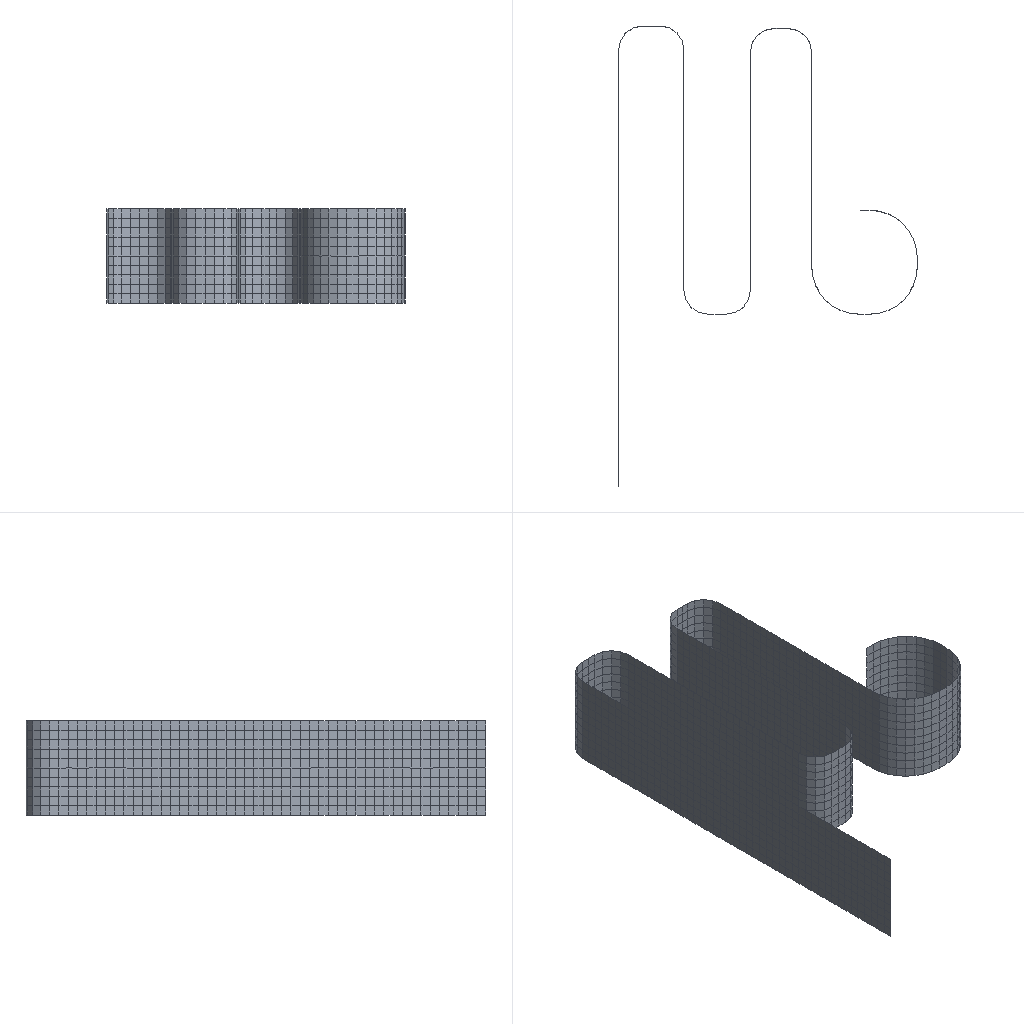Simulation study | ansys workbench
Set-up summary:
category,name,step,type,value,unit,region
solver,ansys_workbench
units,mm-N-s-tonne (MPa),,stated,"/units,MPA"
analysis,deck-1/LS1,,static
load_step,deck-1/LS1,deck-1/LS1,static,nsubst=1; time=1
analysis,deck-2/LS1,,static
load_step,deck-2/LS1,deck-2/LS1,static,nsubst=1; time=1
mesh,deck-1.dat,,nodes,1980
mesh,deck-1.dat,,elements,1800
element_type,SHELL181,,,1790,,deck-1.dat
element_type,SURF156,,,10,,deck-1.dat
mesh,deck-2.dat,,nodes,1980
mesh,deck-2.dat,,elements,1800
element_type,SHELL181,,,1790,,deck-2.dat
element_type,SURF156,,,10,,deck-2.dat
material,Structural steel,,E,200000,tonne s^-2 mm^-1
material,Structural steel,,nu,0.3
material,Structural steel,,density,7.85e-09,tonne mm^-3
material,Structural steel,,conductivity,60.5,tonne mm s^-3 C^-1
material,Structural steel,,specific_heat,4.34e+08,mm^2 s^-2 C^-1
material,Structural steel,,cte,1.2e-05,C^-1
material,Structural steel,,permeability,10000
material,Structural steel,,resistivity,0.00017,ohm mm
load,Define Force Using Surface Effect Elements,deck-1/LS1,surface-effect pres face 1,25,,SURF156 #2
load,Define Force Using Surface Effect Elements,deck-2/LS1,surface-effect pres face 1,25,,SURF156 #2
bc,Fixed Supports,deck-1/model,fixed,[dofs=ALL],,_FIXEDSU
bc,Fixed Supports,deck-2/model,fixed,[dofs=ALL],,_FIXEDSU
named_set,_FIXEDSU,,node,11
named_set,_FIXEDSU,,node,11
Results summary:
result,analyses[0].index,,,1
result,analyses[0].system,,,SYS
result,analyses[0].deck,,,deck-1.dat
result,analyses[0].solve_status,,,completed
result,analyses[0].analysis_type,,,static
result,analyses[0].physics,,,mechanical
result,analyses[0].unit_system,,,"NMM: mm, ton, N, s, mV, mA, degC"
result,analyses[0].n_sets,,,1
result,analyses[0].load_steps[0].set,set=1,,1
result,analyses[0].load_steps[0].time_or_freq,set=1,,1
result,analyses[0].load_steps[0].max_displacement_magnitude,set=1,,37.678
result,analyses[0].load_steps[0].max_von_mises_nodal,set=1,,4347.06
result,analyses[0].load_steps[0].reaction_force_sum_xyz[1],set=1,,-250
result,analyses[0].load_steps[0].reaction_force_sum_xyz[2],set=1,,5.09169e-09
result,analyses[0].load_steps[0].reaction_force_sum_xyz[3],set=1,,2.90072e-09
result,analyses[1].index,,,2
result,analyses[1].system,,,SYS-1
result,analyses[1].deck,,,deck-2.dat
result,analyses[1].solve_status,,,completed
result,analyses[1].analysis_type,,,static
result,analyses[1].physics,,,mechanical
result,analyses[1].unit_system,,,"NMM: mm, ton, N, s, mV, mA, degC"
result,analyses[1].n_sets,,,5
result,analyses[1].load_steps[0].set,set=5,,5
result,analyses[1].load_steps[0].time_or_freq,set=5,,1
result,analyses[1].load_steps[0].max_displacement_magnitude,set=5,,31.218
result,analyses[1].load_steps[0].max_von_mises_nodal,set=5,,3865.32
result,analyses[1].load_steps[0].reaction_force_sum_xyz[1],set=5,,-250
result,analyses[1].load_steps[0].reaction_force_sum_xyz[2],set=5,,-0.003967
result,analyses[1].load_steps[0].reaction_force_sum_xyz[3],set=5,,1.17473e-06
result,geometry_export[0][0],,,1.step
result,geometry_export[0][1],,,ok
result,geometry_export[0][2],,,1
result,geometry_export[1][0],,,2.step
result,geometry_export[1][1],,,ok
result,geometry_export[1][2],,,1